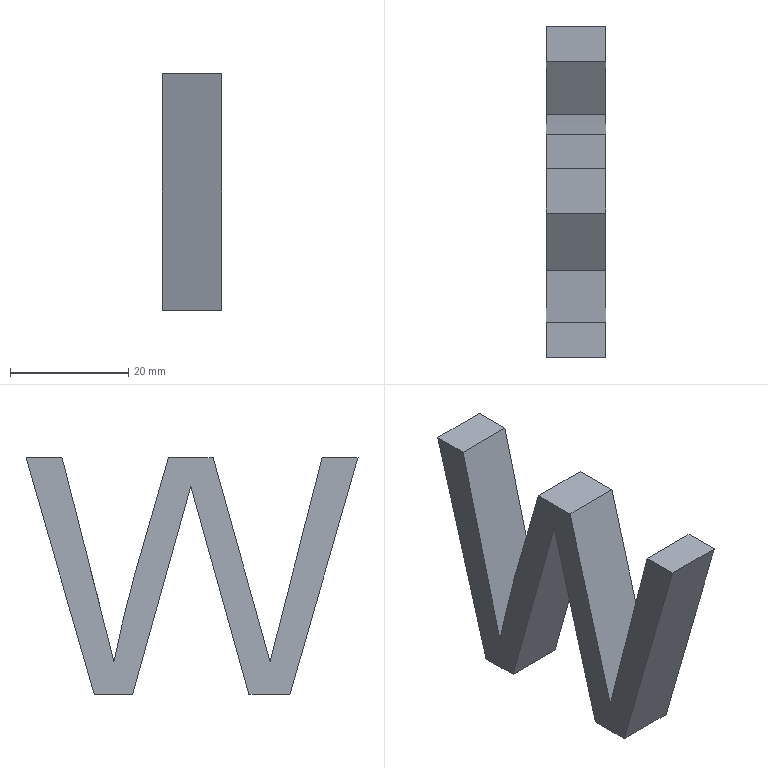Part | NX | features solid 2 | 1 solid | 16 faces | box 10 x 56.061 x 40 mm | volume 8225 mm3 | plane 10 | spline 6
STEP:
#1=CARTESIAN_POINT('',(2250.,284.417,-590.));
#2=VERTEX_POINT('',#1);
#3=CARTESIAN_POINT('',(2250.,277.503,-590.));
#4=VERTEX_POINT('',#3);
#5=CARTESIAN_POINT('',(2250.,284.417,-590.));
#6=CARTESIAN_POINT('',(2250.,282.112,-590.));
#7=CARTESIAN_POINT('',(2250.,279.808,-590.));
#8=CARTESIAN_POINT('',(2250.,277.503,-590.));
#9=B_SPLINE_CURVE_WITH_KNOTS('',3,(#5,#6,#7,#8),.UNSPECIFIED.,.F.,.F.,(4,4),(0.,0.02097),.PIECEWISE_BEZIER_KNOTS.);
#10=EDGE_CURVE('',#2,#4,#9,.T.);
#11=ORIENTED_EDGE('',*,*,#10,.F.);
#12=CARTESIAN_POINT('',(2260.,284.417,-590.));
#13=VERTEX_POINT('',#12);
#14=CARTESIAN_POINT('',(2260.,284.417,-590.));
#15=DIRECTION('',(-1.,0.,0.));
#16=VECTOR('',#15,1000.);
#17=LINE('',#14,#16);
#18=EDGE_CURVE('',#13,#2,#17,.T.);
#19=ORIENTED_EDGE('',*,*,#18,.F.);
#20=CARTESIAN_POINT('',(2260.,277.503,-590.));
#21=VERTEX_POINT('',#20);
#22=CARTESIAN_POINT('',(2260.,284.417,-590.));
#23=CARTESIAN_POINT('',(2260.,282.112,-590.));
#24=CARTESIAN_POINT('',(2260.,279.808,-590.));
#25=CARTESIAN_POINT('',(2260.,277.503,-590.));
#26=B_SPLINE_CURVE_WITH_KNOTS('',3,(#22,#23,#24,#25),.UNSPECIFIED.,.F.,.F.,(4,4),(0.,0.02097),.PIECEWISE_BEZIER_KNOTS.);
#27=EDGE_CURVE('',#13,#21,#26,.T.);
#28=ORIENTED_EDGE('',*,*,#27,.T.);
#29=CARTESIAN_POINT('',(2260.,277.503,-590.));
#30=DIRECTION('',(-1.,0.,0.));
#31=VECTOR('',#30,1000.);
#32=LINE('',#29,#31);
#33=EDGE_CURVE('',#21,#4,#32,.T.);
#34=ORIENTED_EDGE('',*,*,#33,.T.);
#35=EDGE_LOOP('',(#11,#19,#28,#34));
#36=FACE_BOUND('',#35,.T.);
#37=CARTESIAN_POINT('',(2260.,284.417,-590.));
#38=DIRECTION('',(0.,0.,-1.));
#39=DIRECTION('',(-1.,0.,0.));
#40=AXIS2_PLACEMENT_3D('',#37,#38,#39);
#41=PLANE('',#40);
#42=ADVANCED_FACE('',(#36),#41,.T.);
#43=CARTESIAN_POINT('',(2250.,266.,-550.));
#44=VERTEX_POINT('',#43);
#45=CARTESIAN_POINT('',(2250.,277.503,-590.));
#46=CARTESIAN_POINT('',(2250.,273.669,-576.667));
#47=CARTESIAN_POINT('',(2250.,269.834,-563.333));
#48=CARTESIAN_POINT('',(2250.,266.,-550.));
#49=B_SPLINE_CURVE_WITH_KNOTS('',3,(#45,#46,#47,#48),.UNSPECIFIED.,.F.,.F.,(4,4),(0.02097,0.1472),.PIECEWISE_BEZIER_KNOTS.);
#50=EDGE_CURVE('',#4,#44,#49,.T.);
#51=ORIENTED_EDGE('',*,*,#50,.F.);
#52=ORIENTED_EDGE('',*,*,#33,.F.);
#53=CARTESIAN_POINT('',(2260.,266.,-550.));
#54=VERTEX_POINT('',#53);
#55=CARTESIAN_POINT('',(2260.,277.503,-590.));
#56=CARTESIAN_POINT('',(2260.,273.669,-576.667));
#57=CARTESIAN_POINT('',(2260.,269.834,-563.333));
#58=CARTESIAN_POINT('',(2260.,266.,-550.));
#59=B_SPLINE_CURVE_WITH_KNOTS('',3,(#55,#56,#57,#58),.UNSPECIFIED.,.F.,.F.,(4,4),(0.02097,0.1472),.PIECEWISE_BEZIER_KNOTS.);
#60=EDGE_CURVE('',#21,#54,#59,.T.);
#61=ORIENTED_EDGE('',*,*,#60,.T.);
#62=CARTESIAN_POINT('',(2260.,266.,-550.));
#63=DIRECTION('',(-1.,0.,0.));
#64=VECTOR('',#63,1000.);
#65=LINE('',#62,#64);
#66=EDGE_CURVE('',#54,#44,#65,.T.);
#67=ORIENTED_EDGE('',*,*,#66,.T.);
#68=EDGE_LOOP('',(#51,#52,#61,#67));
#69=FACE_BOUND('',#68,.T.);
#70=CARTESIAN_POINT('',(2260.,277.503,-590.));
#71=DIRECTION('',(0.,-0.9611,-0.2764));
#72=DIRECTION('',(0.,0.2764,-0.9611));
#73=AXIS2_PLACEMENT_3D('',#70,#71,#72);
#74=PLANE('',#73);
#75=ADVANCED_FACE('',(#69),#74,.T.);
#76=CARTESIAN_POINT('',(2250.,272.042,-550.));
#77=VERTEX_POINT('',#76);
#78=CARTESIAN_POINT('',(2250.,266.,-550.));
#79=CARTESIAN_POINT('',(2250.,268.014,-550.));
#80=CARTESIAN_POINT('',(2250.,270.028,-550.));
#81=CARTESIAN_POINT('',(2250.,272.042,-550.));
#82=B_SPLINE_CURVE_WITH_KNOTS('',3,(#78,#79,#80,#81),.UNSPECIFIED.,.F.,.F.,(4,4),(0.1472,0.1656),.PIECEWISE_BEZIER_KNOTS.);
#83=EDGE_CURVE('',#44,#77,#82,.T.);
#84=ORIENTED_EDGE('',*,*,#83,.F.);
#85=ORIENTED_EDGE('',*,*,#66,.F.);
#86=CARTESIAN_POINT('',(2260.,272.042,-550.));
#87=VERTEX_POINT('',#86);
#88=CARTESIAN_POINT('',(2260.,266.,-550.));
#89=CARTESIAN_POINT('',(2260.,268.014,-550.));
#90=CARTESIAN_POINT('',(2260.,270.028,-550.));
#91=CARTESIAN_POINT('',(2260.,272.042,-550.));
#92=B_SPLINE_CURVE_WITH_KNOTS('',3,(#88,#89,#90,#91),.UNSPECIFIED.,.F.,.F.,(4,4),(0.1472,0.1656),.PIECEWISE_BEZIER_KNOTS.);
#93=EDGE_CURVE('',#54,#87,#92,.T.);
#94=ORIENTED_EDGE('',*,*,#93,.T.);
#95=CARTESIAN_POINT('',(2260.,272.042,-550.));
#96=DIRECTION('',(-1.,0.,0.));
#97=VECTOR('',#96,1000.);
#98=LINE('',#95,#97);
#99=EDGE_CURVE('',#87,#77,#98,.T.);
#100=ORIENTED_EDGE('',*,*,#99,.T.);
#101=EDGE_LOOP('',(#84,#85,#94,#100));
#102=FACE_BOUND('',#101,.T.);
#103=CARTESIAN_POINT('',(2260.,266.,-550.));
#104=DIRECTION('',(0.,0.,1.));
#105=DIRECTION('',(1.,0.,0.));
#106=AXIS2_PLACEMENT_3D('',#103,#104,#105);
#107=PLANE('',#106);
#108=ADVANCED_FACE('',(#102),#107,.T.);
#109=CARTESIAN_POINT('',(2250.,280.853,-584.417));
#110=VERTEX_POINT('',#109);
#111=CARTESIAN_POINT('',(2250.,272.042,-550.));
#112=CARTESIAN_POINT('',(2250.,274.275,-558.709));
#113=CARTESIAN_POINT('',(2250.,276.509,-567.417));
#114=CARTESIAN_POINT('',(2250.,279.451,-578.893));
#115=CARTESIAN_POINT('',(2250.,280.149,-581.648));
#116=CARTESIAN_POINT('',(2250.,280.853,-584.417));
#117=B_SPLINE_CURVE_WITH_KNOTS('',3,(#111,#112,#113,#114,#115,#116),.UNSPECIFIED.,.F.,.F.,(4,2,4),(0.1656,0.2474,0.2734),.UNSPECIFIED.);
#118=EDGE_CURVE('',#77,#110,#117,.T.);
#119=ORIENTED_EDGE('',*,*,#118,.F.);
#120=ORIENTED_EDGE('',*,*,#99,.F.);
#121=CARTESIAN_POINT('',(2260.,280.853,-584.417));
#122=VERTEX_POINT('',#121);
#123=CARTESIAN_POINT('',(2260.,272.042,-550.));
#124=CARTESIAN_POINT('',(2260.,274.275,-558.709));
#125=CARTESIAN_POINT('',(2260.,276.509,-567.417));
#126=CARTESIAN_POINT('',(2260.,279.451,-578.893));
#127=CARTESIAN_POINT('',(2260.,280.149,-581.648));
#128=CARTESIAN_POINT('',(2260.,280.853,-584.417));
#129=B_SPLINE_CURVE_WITH_KNOTS('',3,(#123,#124,#125,#126,#127,#128),.UNSPECIFIED.,.F.,.F.,(4,2,4),(0.1656,0.2474,0.2734),.UNSPECIFIED.);
#130=EDGE_CURVE('',#87,#122,#129,.T.);
#131=ORIENTED_EDGE('',*,*,#130,.T.);
#132=CARTESIAN_POINT('',(2260.,280.853,-584.417));
#133=DIRECTION('',(-1.,0.,0.));
#134=VECTOR('',#133,1000.);
#135=LINE('',#132,#134);
#136=EDGE_CURVE('',#122,#110,#135,.T.);
#137=ORIENTED_EDGE('',*,*,#136,.T.);
#138=EDGE_LOOP('',(#119,#120,#131,#137));
#139=FACE_BOUND('',#138,.T.);
#140=CARTESIAN_POINT('',(2260.,272.042,-550.));
#141=CARTESIAN_POINT('',(2250.,272.042,-550.));
#142=CARTESIAN_POINT('',(2260.,274.985,-561.476));
#143=CARTESIAN_POINT('',(2250.,274.985,-561.476));
#144=CARTESIAN_POINT('',(2260.,277.935,-572.935));
#145=CARTESIAN_POINT('',(2250.,277.935,-572.935));
#146=CARTESIAN_POINT('',(2260.,280.853,-584.417));
#147=CARTESIAN_POINT('',(2250.,280.853,-584.417));
#148=B_SPLINE_SURFACE_WITH_KNOTS('',3,1,((#140,#141),(#142,#143),(#144,#145),(#146,#147)),.SURF_OF_LINEAR_EXTRUSION.,.F.,.F.,.F.,(4,4),(2,2),(0.1656,0.2734),(0.,1.),.PIECEWISE_BEZIER_KNOTS.);
#149=ADVANCED_FACE('',(#139),#148,.T.);
#150=CARTESIAN_POINT('',(2250.,290.474,-550.));
#151=VERTEX_POINT('',#150);
#152=CARTESIAN_POINT('',(2250.,280.853,-584.417));
#153=CARTESIAN_POINT('',(2250.,282.,-580.302));
#154=CARTESIAN_POINT('',(2250.,282.688,-577.901));
#155=CARTESIAN_POINT('',(2250.,282.879,-577.214));
#156=CARTESIAN_POINT('',(2250.,285.406,-568.141));
#157=CARTESIAN_POINT('',(2250.,287.94,-559.071));
#158=CARTESIAN_POINT('',(2250.,290.474,-550.));
#159=B_SPLINE_CURVE_WITH_KNOTS('',3,(#152,#153,#154,#155,#156,#157,#158),.UNSPECIFIED.,.F.,.F.,(4,3,4),(0.2734,0.2961,0.3818),.PIECEWISE_BEZIER_KNOTS.);
#160=EDGE_CURVE('',#110,#151,#159,.T.);
#161=ORIENTED_EDGE('',*,*,#160,.F.);
#162=ORIENTED_EDGE('',*,*,#136,.F.);
#163=CARTESIAN_POINT('',(2260.,290.474,-550.));
#164=VERTEX_POINT('',#163);
#165=CARTESIAN_POINT('',(2260.,280.853,-584.417));
#166=CARTESIAN_POINT('',(2260.,282.,-580.302));
#167=CARTESIAN_POINT('',(2260.,282.688,-577.901));
#168=CARTESIAN_POINT('',(2260.,282.879,-577.214));
#169=CARTESIAN_POINT('',(2260.,285.406,-568.141));
#170=CARTESIAN_POINT('',(2260.,287.94,-559.071));
#171=CARTESIAN_POINT('',(2260.,290.474,-550.));
#172=B_SPLINE_CURVE_WITH_KNOTS('',3,(#165,#166,#167,#168,#169,#170,#171),.UNSPECIFIED.,.F.,.F.,(4,3,4),(0.2734,0.2961,0.3818),.PIECEWISE_BEZIER_KNOTS.);
#173=EDGE_CURVE('',#122,#164,#172,.T.);
#174=ORIENTED_EDGE('',*,*,#173,.T.);
#175=CARTESIAN_POINT('',(2260.,290.474,-550.));
#176=DIRECTION('',(-1.,0.,0.));
#177=VECTOR('',#176,1000.);
#178=LINE('',#175,#177);
#179=EDGE_CURVE('',#164,#151,#178,.T.);
#180=ORIENTED_EDGE('',*,*,#179,.T.);
#181=EDGE_LOOP('',(#161,#162,#174,#180));
#182=FACE_BOUND('',#181,.T.);
#183=CARTESIAN_POINT('',(2260.,280.853,-584.417));
#184=CARTESIAN_POINT('',(2250.,280.853,-584.417));
#185=CARTESIAN_POINT('',(2260.,281.195,-583.189));
#186=CARTESIAN_POINT('',(2250.,281.195,-583.189));
#187=CARTESIAN_POINT('',(2260.,281.798,-581.037));
#188=CARTESIAN_POINT('',(2250.,281.798,-581.037));
#189=CARTESIAN_POINT('',(2260.,282.343,-579.112));
#190=CARTESIAN_POINT('',(2250.,282.343,-579.112));
#191=CARTESIAN_POINT('',(2260.,282.65,-578.029));
#192=CARTESIAN_POINT('',(2250.,282.65,-578.029));
#193=CARTESIAN_POINT('',(2260.,282.786,-577.546));
#194=CARTESIAN_POINT('',(2250.,282.786,-577.546));
#195=CARTESIAN_POINT('',(2260.,282.855,-577.303));
#196=CARTESIAN_POINT('',(2250.,282.855,-577.303));
#197=CARTESIAN_POINT('',(2260.,282.883,-577.2));
#198=CARTESIAN_POINT('',(2250.,282.883,-577.2));
#199=CARTESIAN_POINT('',(2260.,283.001,-576.779));
#200=CARTESIAN_POINT('',(2250.,283.001,-576.779));
#201=CARTESIAN_POINT('',(2260.,283.117,-576.361));
#202=CARTESIAN_POINT('',(2250.,283.117,-576.361));
#203=CARTESIAN_POINT('',(2260.,283.32,-575.632));
#204=CARTESIAN_POINT('',(2250.,283.32,-575.632));
#205=CARTESIAN_POINT('',(2260.,283.568,-574.741));
#206=CARTESIAN_POINT('',(2250.,283.568,-574.741));
#207=CARTESIAN_POINT('',(2260.,283.969,-573.305));
#208=CARTESIAN_POINT('',(2250.,283.969,-573.305));
#209=CARTESIAN_POINT('',(2260.,284.468,-571.513));
#210=CARTESIAN_POINT('',(2250.,284.468,-571.513));
#211=CARTESIAN_POINT('',(2260.,285.068,-569.361));
#212=CARTESIAN_POINT('',(2250.,285.068,-569.361));
#213=CARTESIAN_POINT('',(2260.,285.868,-566.493));
#214=CARTESIAN_POINT('',(2250.,285.868,-566.493));
#215=CARTESIAN_POINT('',(2260.,286.869,-562.907));
#216=CARTESIAN_POINT('',(2250.,286.869,-562.907));
#217=CARTESIAN_POINT('',(2260.,288.471,-557.171));
#218=CARTESIAN_POINT('',(2250.,288.471,-557.171));
#219=CARTESIAN_POINT('',(2260.,289.673,-552.868));
#220=CARTESIAN_POINT('',(2250.,289.673,-552.868));
#221=CARTESIAN_POINT('',(2260.,290.474,-550.));
#222=CARTESIAN_POINT('',(2250.,290.474,-550.));
#223=B_SPLINE_SURFACE_WITH_KNOTS('',3,1,((#183,#184),(#185,#186),(#187,#188),(#189,#190),(#191,#192),(#193,#194),(#195,#196),(#197,#198),(#199,#200),(#201,#202),(#203,#204),(#205,#206),(#207,#208),(#209,#210),(#211,#212),(#213,#214),(#215,#216),(#217,#218),(#219,#220),(#221,#222)),.SURF_OF_LINEAR_EXTRUSION.,.F.,.F.,.F.,(4,1,1,1,1,1,1,1,1,1,1,1,1,1,1,1,1,4),(2,2),(0.2734,0.2802,0.2869,0.2903,0.2937,0.2954,0.2963,0.2971,0.2988,0.3005,0.3039,0.3073,0.314,0.3208,0.3276,0.3411,0.3547,0.3818),(0.,1.),.UNSPECIFIED.);
#224=ADVANCED_FACE('',(#182),#223,.T.);
#225=CARTESIAN_POINT('',(2250.,298.,-550.));
#226=VERTEX_POINT('',#225);
#227=CARTESIAN_POINT('',(2250.,290.474,-550.));
#228=CARTESIAN_POINT('',(2250.,292.983,-550.));
#229=CARTESIAN_POINT('',(2250.,295.491,-550.));
#230=CARTESIAN_POINT('',(2250.,298.,-550.));
#231=B_SPLINE_CURVE_WITH_KNOTS('',3,(#227,#228,#229,#230),.UNSPECIFIED.,.F.,.F.,(4,4),(0.3818,0.4046),.PIECEWISE_BEZIER_KNOTS.);
#232=EDGE_CURVE('',#151,#226,#231,.T.);
#233=ORIENTED_EDGE('',*,*,#232,.F.);
#234=ORIENTED_EDGE('',*,*,#179,.F.);
#235=CARTESIAN_POINT('',(2260.,298.,-550.));
#236=VERTEX_POINT('',#235);
#237=CARTESIAN_POINT('',(2260.,290.474,-550.));
#238=CARTESIAN_POINT('',(2260.,292.983,-550.));
#239=CARTESIAN_POINT('',(2260.,295.491,-550.));
#240=CARTESIAN_POINT('',(2260.,298.,-550.));
#241=B_SPLINE_CURVE_WITH_KNOTS('',3,(#237,#238,#239,#240),.UNSPECIFIED.,.F.,.F.,(4,4),(0.3818,0.4046),.PIECEWISE_BEZIER_KNOTS.);
#242=EDGE_CURVE('',#164,#236,#241,.T.);
#243=ORIENTED_EDGE('',*,*,#242,.T.);
#244=CARTESIAN_POINT('',(2260.,298.,-550.));
#245=DIRECTION('',(-1.,0.,0.));
#246=VECTOR('',#245,1000.);
#247=LINE('',#244,#246);
#248=EDGE_CURVE('',#236,#226,#247,.T.);
#249=ORIENTED_EDGE('',*,*,#248,.T.);
#250=EDGE_LOOP('',(#233,#234,#243,#249));
#251=FACE_BOUND('',#250,.T.);
#252=CARTESIAN_POINT('',(2260.,290.474,-550.));
#253=DIRECTION('',(0.,0.,1.));
#254=DIRECTION('',(1.,0.,0.));
#255=AXIS2_PLACEMENT_3D('',#252,#253,#254);
#256=PLANE('',#255);
#257=ADVANCED_FACE('',(#251),#256,.T.);
#258=CARTESIAN_POINT('',(2250.,303.813,-570.13));
#259=VERTEX_POINT('',#258);
#260=CARTESIAN_POINT('',(2250.,298.,-550.));
#261=CARTESIAN_POINT('',(2250.,299.938,-556.71));
#262=CARTESIAN_POINT('',(2250.,301.875,-563.42));
#263=CARTESIAN_POINT('',(2250.,303.813,-570.13));
#264=B_SPLINE_CURVE_WITH_KNOTS('',3,(#260,#261,#262,#263),.UNSPECIFIED.,.F.,.F.,(4,4),(0.4046,0.4682),.PIECEWISE_BEZIER_KNOTS.);
#265=EDGE_CURVE('',#226,#259,#264,.T.);
#266=ORIENTED_EDGE('',*,*,#265,.F.);
#267=ORIENTED_EDGE('',*,*,#248,.F.);
#268=CARTESIAN_POINT('',(2260.,303.813,-570.13));
#269=VERTEX_POINT('',#268);
#270=CARTESIAN_POINT('',(2260.,298.,-550.));
#271=CARTESIAN_POINT('',(2260.,299.938,-556.71));
#272=CARTESIAN_POINT('',(2260.,301.875,-563.42));
#273=CARTESIAN_POINT('',(2260.,303.813,-570.13));
#274=B_SPLINE_CURVE_WITH_KNOTS('',3,(#270,#271,#272,#273),.UNSPECIFIED.,.F.,.F.,(4,4),(0.4046,0.4682),.PIECEWISE_BEZIER_KNOTS.);
#275=EDGE_CURVE('',#236,#269,#274,.T.);
#276=ORIENTED_EDGE('',*,*,#275,.T.);
#277=CARTESIAN_POINT('',(2260.,303.813,-570.13));
#278=DIRECTION('',(-1.,0.,0.));
#279=VECTOR('',#278,1000.);
#280=LINE('',#277,#279);
#281=EDGE_CURVE('',#269,#259,#280,.T.);
#282=ORIENTED_EDGE('',*,*,#281,.T.);
#283=EDGE_LOOP('',(#266,#267,#276,#282));
#284=FACE_BOUND('',#283,.T.);
#285=CARTESIAN_POINT('',(2260.,298.,-550.));
#286=DIRECTION('',(0.,0.9607,0.2774));
#287=DIRECTION('',(0.,-0.2774,0.9607));
#288=AXIS2_PLACEMENT_3D('',#285,#286,#287);
#289=PLANE('',#288);
#290=ADVANCED_FACE('',(#284),#289,.T.);
#291=CARTESIAN_POINT('',(2250.,307.208,-584.417));
#292=VERTEX_POINT('',#291);
#293=CARTESIAN_POINT('',(2250.,303.813,-570.13));
#294=CARTESIAN_POINT('',(2250.,305.159,-575.224));
#295=CARTESIAN_POINT('',(2250.,306.321,-580.011));
#296=CARTESIAN_POINT('',(2250.,307.208,-584.417));
#297=B_SPLINE_CURVE_WITH_KNOTS('',3,(#293,#294,#295,#296),.UNSPECIFIED.,.F.,.F.,(4,4),(0.4682,0.5128),.PIECEWISE_BEZIER_KNOTS.);
#298=EDGE_CURVE('',#259,#292,#297,.T.);
#299=ORIENTED_EDGE('',*,*,#298,.F.);
#300=ORIENTED_EDGE('',*,*,#281,.F.);
#301=CARTESIAN_POINT('',(2260.,307.208,-584.417));
#302=VERTEX_POINT('',#301);
#303=CARTESIAN_POINT('',(2260.,303.813,-570.13));
#304=CARTESIAN_POINT('',(2260.,305.159,-575.224));
#305=CARTESIAN_POINT('',(2260.,306.321,-580.011));
#306=CARTESIAN_POINT('',(2260.,307.208,-584.417));
#307=B_SPLINE_CURVE_WITH_KNOTS('',3,(#303,#304,#305,#306),.UNSPECIFIED.,.F.,.F.,(4,4),(0.4682,0.5128),.PIECEWISE_BEZIER_KNOTS.);
#308=EDGE_CURVE('',#269,#302,#307,.T.);
#309=ORIENTED_EDGE('',*,*,#308,.T.);
#310=CARTESIAN_POINT('',(2260.,307.208,-584.417));
#311=DIRECTION('',(-1.,0.,0.));
#312=VECTOR('',#311,1000.);
#313=LINE('',#310,#312);
#314=EDGE_CURVE('',#302,#292,#313,.T.);
#315=ORIENTED_EDGE('',*,*,#314,.T.);
#316=EDGE_LOOP('',(#299,#300,#309,#315));
#317=FACE_BOUND('',#316,.T.);
#318=CARTESIAN_POINT('',(2260.,303.813,-570.13));
#319=CARTESIAN_POINT('',(2250.,303.813,-570.13));
#320=CARTESIAN_POINT('',(2260.,305.159,-575.224));
#321=CARTESIAN_POINT('',(2250.,305.159,-575.224));
#322=CARTESIAN_POINT('',(2260.,306.321,-580.011));
#323=CARTESIAN_POINT('',(2250.,306.321,-580.011));
#324=CARTESIAN_POINT('',(2260.,307.208,-584.417));
#325=CARTESIAN_POINT('',(2250.,307.208,-584.417));
#326=B_SPLINE_SURFACE_WITH_KNOTS('',3,1,((#318,#319),(#320,#321),(#322,#323),(#324,#325)),.SURF_OF_LINEAR_EXTRUSION.,.F.,.F.,.F.,(4,4),(2,2),(0.4682,0.5128),(0.,1.),.PIECEWISE_BEZIER_KNOTS.);
#327=ADVANCED_FACE('',(#317),#326,.T.);
#328=CARTESIAN_POINT('',(2250.,315.989,-550.));
#329=VERTEX_POINT('',#328);
#330=CARTESIAN_POINT('',(2250.,307.208,-584.417));
#331=CARTESIAN_POINT('',(2250.,307.836,-582.));
#332=CARTESIAN_POINT('',(2250.,308.57,-579.124));
#333=CARTESIAN_POINT('',(2250.,311.561,-567.215));
#334=CARTESIAN_POINT('',(2250.,313.791,-558.612));
#335=CARTESIAN_POINT('',(2250.,315.989,-550.));
#336=B_SPLINE_CURVE_WITH_KNOTS('',3,(#330,#331,#332,#333,#334,#335),.UNSPECIFIED.,.F.,.F.,(4,2,4),(0.5128,0.5396,0.6101),.UNSPECIFIED.);
#337=EDGE_CURVE('',#292,#329,#336,.T.);
#338=ORIENTED_EDGE('',*,*,#337,.F.);
#339=ORIENTED_EDGE('',*,*,#314,.F.);
#340=CARTESIAN_POINT('',(2260.,315.989,-550.));
#341=VERTEX_POINT('',#340);
#342=CARTESIAN_POINT('',(2260.,307.208,-584.417));
#343=CARTESIAN_POINT('',(2260.,307.836,-582.));
#344=CARTESIAN_POINT('',(2260.,308.57,-579.124));
#345=CARTESIAN_POINT('',(2260.,311.561,-567.215));
#346=CARTESIAN_POINT('',(2260.,313.791,-558.612));
#347=CARTESIAN_POINT('',(2260.,315.989,-550.));
#348=B_SPLINE_CURVE_WITH_KNOTS('',3,(#342,#343,#344,#345,#346,#347),.UNSPECIFIED.,.F.,.F.,(4,2,4),(0.5128,0.5396,0.6101),.UNSPECIFIED.);
#349=EDGE_CURVE('',#302,#341,#348,.T.);
#350=ORIENTED_EDGE('',*,*,#349,.T.);
#351=CARTESIAN_POINT('',(2260.,315.989,-550.));
#352=DIRECTION('',(-1.,0.,0.));
#353=VECTOR('',#352,1000.);
#354=LINE('',#351,#353);
#355=EDGE_CURVE('',#341,#329,#354,.T.);
#356=ORIENTED_EDGE('',*,*,#355,.T.);
#357=EDGE_LOOP('',(#338,#339,#350,#356));
#358=FACE_BOUND('',#357,.T.);
#359=CARTESIAN_POINT('',(2260.,307.208,-584.417));
#360=CARTESIAN_POINT('',(2250.,307.208,-584.417));
#361=CARTESIAN_POINT('',(2260.,307.492,-583.323));
#362=CARTESIAN_POINT('',(2250.,307.492,-583.323));
#363=CARTESIAN_POINT('',(2260.,308.103,-580.952));
#364=CARTESIAN_POINT('',(2250.,308.103,-580.952));
#365=CARTESIAN_POINT('',(2260.,309.148,-576.828));
#366=CARTESIAN_POINT('',(2250.,309.148,-576.828));
#367=CARTESIAN_POINT('',(2260.,310.288,-572.289));
#368=CARTESIAN_POINT('',(2250.,310.288,-572.289));
#369=CARTESIAN_POINT('',(2260.,311.796,-566.364));
#370=CARTESIAN_POINT('',(2250.,311.796,-566.364));
#371=CARTESIAN_POINT('',(2260.,313.704,-558.918));
#372=CARTESIAN_POINT('',(2250.,313.704,-558.918));
#373=CARTESIAN_POINT('',(2260.,315.23,-552.974));
#374=CARTESIAN_POINT('',(2250.,315.23,-552.974));
#375=CARTESIAN_POINT('',(2260.,315.989,-550.));
#376=CARTESIAN_POINT('',(2250.,315.989,-550.));
#377=B_SPLINE_SURFACE_WITH_KNOTS('',3,1,((#359,#360),(#361,#362),(#363,#364),(#365,#366),(#367,#368),(#369,#370),(#371,#372),(#373,#374),(#375,#376)),.SURF_OF_LINEAR_EXTRUSION.,.F.,.F.,.F.,(4,1,1,1,1,1,4),(2,2),(0.5128,0.5249,0.5371,0.5493,0.5614,0.5857,0.6101),(0.,1.),.UNSPECIFIED.);
#378=ADVANCED_FACE('',(#358),#377,.T.);
#379=CARTESIAN_POINT('',(2250.,322.061,-550.));
#380=VERTEX_POINT('',#379);
#381=CARTESIAN_POINT('',(2250.,315.989,-550.));
#382=CARTESIAN_POINT('',(2250.,318.013,-550.));
#383=CARTESIAN_POINT('',(2250.,320.037,-550.));
#384=CARTESIAN_POINT('',(2250.,322.061,-550.));
#385=B_SPLINE_CURVE_WITH_KNOTS('',3,(#381,#382,#383,#384),.UNSPECIFIED.,.F.,.F.,(4,4),(0.6101,0.6282),.PIECEWISE_BEZIER_KNOTS.);
#386=EDGE_CURVE('',#329,#380,#385,.T.);
#387=ORIENTED_EDGE('',*,*,#386,.F.);
#388=ORIENTED_EDGE('',*,*,#355,.F.);
#389=CARTESIAN_POINT('',(2260.,322.061,-550.));
#390=VERTEX_POINT('',#389);
#391=CARTESIAN_POINT('',(2260.,315.989,-550.));
#392=CARTESIAN_POINT('',(2260.,318.013,-550.));
#393=CARTESIAN_POINT('',(2260.,320.037,-550.));
#394=CARTESIAN_POINT('',(2260.,322.061,-550.));
#395=B_SPLINE_CURVE_WITH_KNOTS('',3,(#391,#392,#393,#394),.UNSPECIFIED.,.F.,.F.,(4,4),(0.6101,0.6282),.PIECEWISE_BEZIER_KNOTS.);
#396=EDGE_CURVE('',#341,#390,#395,.T.);
#397=ORIENTED_EDGE('',*,*,#396,.T.);
#398=CARTESIAN_POINT('',(2260.,322.061,-550.));
#399=DIRECTION('',(-1.,0.,0.));
#400=VECTOR('',#399,1000.);
#401=LINE('',#398,#400);
#402=EDGE_CURVE('',#390,#380,#401,.T.);
#403=ORIENTED_EDGE('',*,*,#402,.T.);
#404=EDGE_LOOP('',(#387,#388,#397,#403));
#405=FACE_BOUND('',#404,.T.);
#406=CARTESIAN_POINT('',(2260.,315.989,-550.));
#407=DIRECTION('',(0.,0.,1.));
#408=DIRECTION('',(1.,0.,0.));
#409=AXIS2_PLACEMENT_3D('',#406,#407,#408);
#410=PLANE('',#409);
#411=ADVANCED_FACE('',(#405),#410,.T.);
#412=CARTESIAN_POINT('',(2250.,310.528,-590.));
#413=VERTEX_POINT('',#412);
#414=CARTESIAN_POINT('',(2250.,322.061,-550.));
#415=CARTESIAN_POINT('',(2250.,318.217,-563.333));
#416=CARTESIAN_POINT('',(2250.,314.372,-576.667));
#417=CARTESIAN_POINT('',(2250.,310.528,-590.));
#418=B_SPLINE_CURVE_WITH_KNOTS('',3,(#414,#415,#416,#417),.UNSPECIFIED.,.F.,.F.,(4,4),(0.6282,0.7524),.PIECEWISE_BEZIER_KNOTS.);
#419=EDGE_CURVE('',#380,#413,#418,.T.);
#420=ORIENTED_EDGE('',*,*,#419,.F.);
#421=ORIENTED_EDGE('',*,*,#402,.F.);
#422=CARTESIAN_POINT('',(2260.,310.528,-590.));
#423=VERTEX_POINT('',#422);
#424=CARTESIAN_POINT('',(2260.,322.061,-550.));
#425=CARTESIAN_POINT('',(2260.,318.217,-563.333));
#426=CARTESIAN_POINT('',(2260.,314.372,-576.667));
#427=CARTESIAN_POINT('',(2260.,310.528,-590.));
#428=B_SPLINE_CURVE_WITH_KNOTS('',3,(#424,#425,#426,#427),.UNSPECIFIED.,.F.,.F.,(4,4),(0.6282,0.7524),.PIECEWISE_BEZIER_KNOTS.);
#429=EDGE_CURVE('',#390,#423,#428,.T.);
#430=ORIENTED_EDGE('',*,*,#429,.T.);
#431=CARTESIAN_POINT('',(2260.,310.528,-590.));
#432=DIRECTION('',(-1.,0.,0.));
#433=VECTOR('',#432,1000.);
#434=LINE('',#431,#433);
#435=EDGE_CURVE('',#423,#413,#434,.T.);
#436=ORIENTED_EDGE('',*,*,#435,.T.);
#437=EDGE_LOOP('',(#420,#421,#430,#436));
#438=FACE_BOUND('',#437,.T.);
#439=CARTESIAN_POINT('',(2260.,322.061,-550.));
#440=DIRECTION('',(0.,0.9609,-0.277));
#441=DIRECTION('',(0.,0.277,0.9609));
#442=AXIS2_PLACEMENT_3D('',#439,#440,#441);
#443=PLANE('',#442);
#444=ADVANCED_FACE('',(#438),#443,.T.);
#445=CARTESIAN_POINT('',(2250.,304.073,-590.));
#446=VERTEX_POINT('',#445);
#447=CARTESIAN_POINT('',(2250.,310.528,-590.));
#448=CARTESIAN_POINT('',(2250.,308.376,-590.));
#449=CARTESIAN_POINT('',(2250.,306.224,-590.));
#450=CARTESIAN_POINT('',(2250.,304.073,-590.));
#451=B_SPLINE_CURVE_WITH_KNOTS('',3,(#447,#448,#449,#450),.UNSPECIFIED.,.F.,.F.,(4,4),(0.7524,0.7716),.PIECEWISE_BEZIER_KNOTS.);
#452=EDGE_CURVE('',#413,#446,#451,.T.);
#453=ORIENTED_EDGE('',*,*,#452,.F.);
#454=ORIENTED_EDGE('',*,*,#435,.F.);
#455=CARTESIAN_POINT('',(2260.,304.073,-590.));
#456=VERTEX_POINT('',#455);
#457=CARTESIAN_POINT('',(2260.,310.528,-590.));
#458=CARTESIAN_POINT('',(2260.,308.376,-590.));
#459=CARTESIAN_POINT('',(2260.,306.224,-590.));
#460=CARTESIAN_POINT('',(2260.,304.073,-590.));
#461=B_SPLINE_CURVE_WITH_KNOTS('',3,(#457,#458,#459,#460),.UNSPECIFIED.,.F.,.F.,(4,4),(0.7524,0.7716),.PIECEWISE_BEZIER_KNOTS.);
#462=EDGE_CURVE('',#423,#456,#461,.T.);
#463=ORIENTED_EDGE('',*,*,#462,.T.);
#464=CARTESIAN_POINT('',(2260.,304.073,-590.));
#465=DIRECTION('',(-1.,0.,0.));
#466=VECTOR('',#465,1000.);
#467=LINE('',#464,#466);
#468=EDGE_CURVE('',#456,#446,#467,.T.);
#469=ORIENTED_EDGE('',*,*,#468,.T.);
#470=EDGE_LOOP('',(#453,#454,#463,#469));
#471=FACE_BOUND('',#470,.T.);
#472=CARTESIAN_POINT('',(2260.,310.528,-590.));
#473=DIRECTION('',(0.,0.,-1.));
#474=DIRECTION('',(-1.,0.,0.));
#475=AXIS2_PLACEMENT_3D('',#472,#473,#474);
#476=PLANE('',#475);
#477=ADVANCED_FACE('',(#471),#476,.T.);
#478=CARTESIAN_POINT('',(2250.,294.237,-554.834));
#479=VERTEX_POINT('',#478);
#480=CARTESIAN_POINT('',(2250.,304.073,-590.));
#481=CARTESIAN_POINT('',(2250.,301.212,-579.792));
#482=CARTESIAN_POINT('',(2250.,298.352,-569.584));
#483=CARTESIAN_POINT('',(2250.,294.784,-556.854));
#484=CARTESIAN_POINT('',(2250.,294.375,-555.323));
#485=CARTESIAN_POINT('',(2250.,294.237,-554.834));
#486=B_SPLINE_CURVE_WITH_KNOTS('',3,(#480,#481,#482,#483,#484,#485),.UNSPECIFIED.,.F.,.F.,(4,2,4),(0.7716,0.8665,0.8899),.UNSPECIFIED.);
#487=EDGE_CURVE('',#446,#479,#486,.T.);
#488=ORIENTED_EDGE('',*,*,#487,.F.);
#489=ORIENTED_EDGE('',*,*,#468,.F.);
#490=CARTESIAN_POINT('',(2260.,294.237,-554.834));
#491=VERTEX_POINT('',#490);
#492=CARTESIAN_POINT('',(2260.,304.073,-590.));
#493=CARTESIAN_POINT('',(2260.,301.212,-579.792));
#494=CARTESIAN_POINT('',(2260.,298.352,-569.584));
#495=CARTESIAN_POINT('',(2260.,294.784,-556.854));
#496=CARTESIAN_POINT('',(2260.,294.375,-555.323));
#497=CARTESIAN_POINT('',(2260.,294.237,-554.834));
#498=B_SPLINE_CURVE_WITH_KNOTS('',3,(#492,#493,#494,#495,#496,#497),.UNSPECIFIED.,.F.,.F.,(4,2,4),(0.7716,0.8665,0.8899),.UNSPECIFIED.);
#499=EDGE_CURVE('',#456,#491,#498,.T.);
#500=ORIENTED_EDGE('',*,*,#499,.T.);
#501=CARTESIAN_POINT('',(2260.,294.237,-554.834));
#502=DIRECTION('',(-1.,0.,0.));
#503=VECTOR('',#502,1000.);
#504=LINE('',#501,#503);
#505=EDGE_CURVE('',#491,#479,#504,.T.);
#506=ORIENTED_EDGE('',*,*,#505,.T.);
#507=EDGE_LOOP('',(#488,#489,#500,#506));
#508=FACE_BOUND('',#507,.T.);
#509=CARTESIAN_POINT('',(2260.,304.073,-590.));
#510=CARTESIAN_POINT('',(2250.,304.073,-590.));
#511=CARTESIAN_POINT('',(2260.,303.181,-586.817));
#512=CARTESIAN_POINT('',(2250.,303.181,-586.817));
#513=CARTESIAN_POINT('',(2260.,301.396,-580.449));
#514=CARTESIAN_POINT('',(2250.,301.396,-580.449));
#515=CARTESIAN_POINT('',(2260.,299.17,-572.503));
#516=CARTESIAN_POINT('',(2250.,299.17,-572.503));
#517=CARTESIAN_POINT('',(2260.,297.38,-566.117));
#518=CARTESIAN_POINT('',(2250.,297.38,-566.117));
#519=CARTESIAN_POINT('',(2260.,296.28,-562.189));
#520=CARTESIAN_POINT('',(2250.,296.28,-562.189));
#521=CARTESIAN_POINT('',(2260.,295.358,-558.903));
#522=CARTESIAN_POINT('',(2250.,295.358,-558.903));
#523=CARTESIAN_POINT('',(2260.,294.612,-556.212));
#524=CARTESIAN_POINT('',(2250.,294.612,-556.212));
#525=CARTESIAN_POINT('',(2260.,294.324,-555.142));
#526=CARTESIAN_POINT('',(2250.,294.324,-555.142));
#527=CARTESIAN_POINT('',(2260.,294.237,-554.834));
#528=CARTESIAN_POINT('',(2250.,294.237,-554.834));
#529=B_SPLINE_SURFACE_WITH_KNOTS('',3,1,((#509,#510),(#511,#512),(#513,#514),(#515,#516),(#517,#518),(#519,#520),(#521,#522),(#523,#524),(#525,#526),(#527,#528)),.SURF_OF_LINEAR_EXTRUSION.,.F.,.F.,.F.,(4,1,1,1,1,1,1,4),(2,2),(0.7716,0.8012,0.8308,0.8456,0.8604,0.8677,0.8751,0.8899),(0.,1.),.UNSPECIFIED.);
#530=ADVANCED_FACE('',(#508),#529,.T.);
#531=CARTESIAN_POINT('',(2250.,294.237,-554.834));
#532=CARTESIAN_POINT('',(2250.,293.717,-556.776));
#533=CARTESIAN_POINT('',(2250.,293.243,-558.382));
#534=CARTESIAN_POINT('',(2250.,292.89,-559.641));
#535=CARTESIAN_POINT('',(2250.,290.056,-569.758));
#536=CARTESIAN_POINT('',(2250.,287.236,-579.879));
#537=CARTESIAN_POINT('',(2250.,284.417,-590.));
#538=B_SPLINE_CURVE_WITH_KNOTS('',3,(#531,#532,#533,#534,#535,#536,#537),.UNSPECIFIED.,.F.,.F.,(4,3,4),(0.8899,0.905,1.),.PIECEWISE_BEZIER_KNOTS.);
#539=EDGE_CURVE('',#479,#2,#538,.T.);
#540=ORIENTED_EDGE('',*,*,#539,.F.);
#541=ORIENTED_EDGE('',*,*,#505,.F.);
#542=CARTESIAN_POINT('',(2260.,294.237,-554.834));
#543=CARTESIAN_POINT('',(2260.,293.717,-556.776));
#544=CARTESIAN_POINT('',(2260.,293.243,-558.382));
#545=CARTESIAN_POINT('',(2260.,292.89,-559.641));
#546=CARTESIAN_POINT('',(2260.,290.056,-569.758));
#547=CARTESIAN_POINT('',(2260.,287.236,-579.879));
#548=CARTESIAN_POINT('',(2260.,284.417,-590.));
#549=B_SPLINE_CURVE_WITH_KNOTS('',3,(#542,#543,#544,#545,#546,#547,#548),.UNSPECIFIED.,.F.,.F.,(4,3,4),(0.8899,0.905,1.),.PIECEWISE_BEZIER_KNOTS.);
#550=EDGE_CURVE('',#491,#13,#549,.T.);
#551=ORIENTED_EDGE('',*,*,#550,.T.);
#552=ORIENTED_EDGE('',*,*,#18,.T.);
#553=EDGE_LOOP('',(#540,#541,#551,#552));
#554=FACE_BOUND('',#553,.T.);
#555=CARTESIAN_POINT('',(2260.,294.237,-554.834));
#556=CARTESIAN_POINT('',(2250.,294.237,-554.834));
#557=CARTESIAN_POINT('',(2260.,293.999,-555.722));
#558=CARTESIAN_POINT('',(2250.,293.999,-555.722));
#559=CARTESIAN_POINT('',(2260.,293.657,-556.948));
#560=CARTESIAN_POINT('',(2250.,293.657,-556.948));
#561=CARTESIAN_POINT('',(2260.,293.251,-558.37));
#562=CARTESIAN_POINT('',(2250.,293.251,-558.37));
#563=CARTESIAN_POINT('',(2260.,293.024,-559.166));
#564=CARTESIAN_POINT('',(2250.,293.024,-559.166));
#565=CARTESIAN_POINT('',(2260.,292.858,-559.756));
#566=CARTESIAN_POINT('',(2250.,292.858,-559.756));
#567=CARTESIAN_POINT('',(2260.,292.643,-560.523));
#568=CARTESIAN_POINT('',(2250.,292.643,-560.523));
#569=CARTESIAN_POINT('',(2260.,292.29,-561.783));
#570=CARTESIAN_POINT('',(2250.,292.29,-561.783));
#571=CARTESIAN_POINT('',(2260.,291.569,-564.362));
#572=CARTESIAN_POINT('',(2250.,291.569,-564.362));
#573=CARTESIAN_POINT('',(2260.,290.547,-568.017));
#574=CARTESIAN_POINT('',(2250.,290.547,-568.017));
#575=CARTESIAN_POINT('',(2260.,288.909,-573.881));
#576=CARTESIAN_POINT('',(2250.,288.909,-573.881));
#577=CARTESIAN_POINT('',(2260.,286.867,-581.206));
#578=CARTESIAN_POINT('',(2250.,286.867,-581.206));
#579=CARTESIAN_POINT('',(2260.,285.233,-587.069));
#580=CARTESIAN_POINT('',(2250.,285.233,-587.069));
#581=CARTESIAN_POINT('',(2260.,284.417,-590.));
#582=CARTESIAN_POINT('',(2250.,284.417,-590.));
#583=B_SPLINE_SURFACE_WITH_KNOTS('',3,1,((#555,#556),(#557,#558),(#559,#560),(#561,#562),(#563,#564),(#565,#566),(#567,#568),(#569,#570),(#571,#572),(#573,#574),(#575,#576),(#577,#578),(#579,#580),(#581,#582)),.SURF_OF_LINEAR_EXTRUSION.,.F.,.F.,.F.,(4,1,1,1,1,1,1,1,1,1,1,4),(2,2),(0.8899,0.8968,0.9002,0.9037,0.9054,0.9071,0.9106,0.9174,0.9312,0.945,0.9725,1.),(0.,1.),.UNSPECIFIED.);
#584=ADVANCED_FACE('',(#554),#583,.T.);
#585=ORIENTED_EDGE('',*,*,#27,.F.);
#586=ORIENTED_EDGE('',*,*,#550,.F.);
#587=ORIENTED_EDGE('',*,*,#499,.F.);
#588=ORIENTED_EDGE('',*,*,#462,.F.);
#589=ORIENTED_EDGE('',*,*,#429,.F.);
#590=ORIENTED_EDGE('',*,*,#396,.F.);
#591=ORIENTED_EDGE('',*,*,#349,.F.);
#592=ORIENTED_EDGE('',*,*,#308,.F.);
#593=ORIENTED_EDGE('',*,*,#275,.F.);
#594=ORIENTED_EDGE('',*,*,#242,.F.);
#595=ORIENTED_EDGE('',*,*,#173,.F.);
#596=ORIENTED_EDGE('',*,*,#130,.F.);
#597=ORIENTED_EDGE('',*,*,#93,.F.);
#598=ORIENTED_EDGE('',*,*,#60,.F.);
#599=EDGE_LOOP('',(#585,#586,#587,#588,#589,#590,#591,#592,#593,#594,#595,#596,#597,#598));
#600=FACE_BOUND('',#599,.T.);
#601=CARTESIAN_POINT('',(2260.,276.456,-567.214));
#602=DIRECTION('',(1.,0.,0.));
#603=DIRECTION('',(0.,1.,0.));
#604=AXIS2_PLACEMENT_3D('',#601,#602,#603);
#605=PLANE('',#604);
#606=ADVANCED_FACE('',(#600),#605,.T.);
#607=ORIENTED_EDGE('',*,*,#10,.T.);
#608=ORIENTED_EDGE('',*,*,#50,.T.);
#609=ORIENTED_EDGE('',*,*,#83,.T.);
#610=ORIENTED_EDGE('',*,*,#118,.T.);
#611=ORIENTED_EDGE('',*,*,#160,.T.);
#612=ORIENTED_EDGE('',*,*,#232,.T.);
#613=ORIENTED_EDGE('',*,*,#265,.T.);
#614=ORIENTED_EDGE('',*,*,#298,.T.);
#615=ORIENTED_EDGE('',*,*,#337,.T.);
#616=ORIENTED_EDGE('',*,*,#386,.T.);
#617=ORIENTED_EDGE('',*,*,#419,.T.);
#618=ORIENTED_EDGE('',*,*,#452,.T.);
#619=ORIENTED_EDGE('',*,*,#487,.T.);
#620=ORIENTED_EDGE('',*,*,#539,.T.);
#621=EDGE_LOOP('',(#607,#608,#609,#610,#611,#612,#613,#614,#615,#616,#617,#618,#619,#620));
#622=FACE_BOUND('',#621,.T.);
#623=CARTESIAN_POINT('',(2250.,276.456,-567.214));
#624=DIRECTION('',(1.,0.,0.));
#625=DIRECTION('',(0.,1.,0.));
#626=AXIS2_PLACEMENT_3D('',#623,#624,#625);
#627=PLANE('',#626);
#628=ADVANCED_FACE('',(#622),#627,.F.);
#629=CLOSED_SHELL('',(#42,#75,#108,#149,#224,#257,#290,#327,#378,#411,#444,#477,#530,#584,#606,#628));
#630=MANIFOLD_SOLID_BREP('',#629);
#631=(LENGTH_UNIT()NAMED_UNIT(*)SI_UNIT(.MILLI.,.METRE.));
#632=UNCERTAINTY_MEASURE_WITH_UNIT(LENGTH_MEASURE(0.0508),#631,'','');
#633=(NAMED_UNIT(*)PLANE_ANGLE_UNIT()SI_UNIT($,.RADIAN.));
#634=(NAMED_UNIT(*)SI_UNIT($,.STERADIAN.)SOLID_ANGLE_UNIT());
#635=(GEOMETRIC_REPRESENTATION_CONTEXT(3)GLOBAL_UNCERTAINTY_ASSIGNED_CONTEXT((#632))GLOBAL_UNIT_ASSIGNED_CONTEXT((#631,#633,#634))REPRESENTATION_CONTEXT('',''));
#636=ADVANCED_BREP_SHAPE_REPRESENTATION('',(#630),#635);